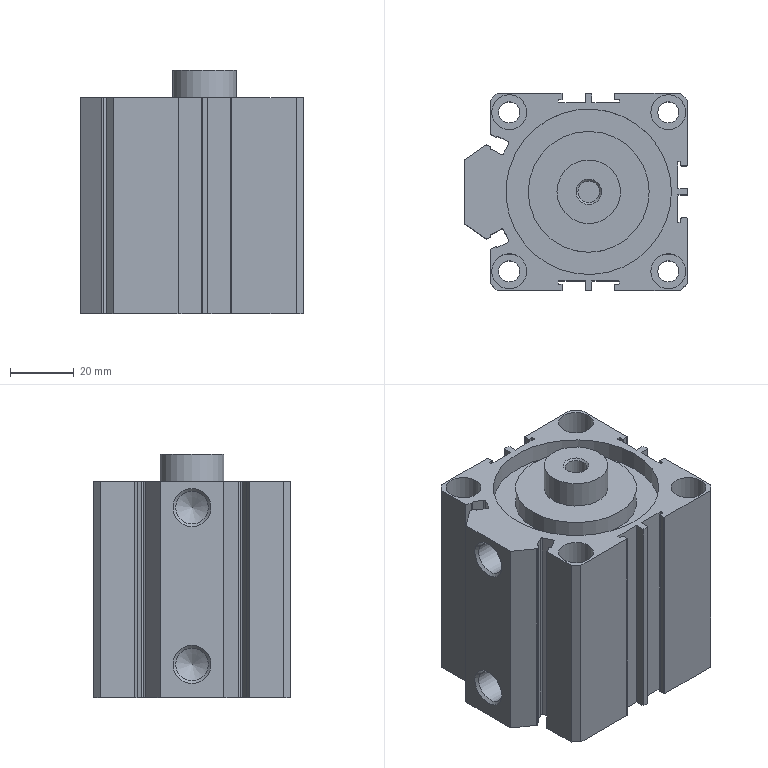Part | NX | features EXTRUDE 7, DATUM_CSYS 5, SKETCH 4, SIMPLE HOLE 3, SYMBOLIC_THREAD 3, HOLE PACKAGE 2 | 2 solids | 142 faces | box 70 x 62 x 76.6 mm | volume 239161 mm3 | plane 73 | cylinder 63 | cone 6 | commonest cylinder face diameters 0.4 x34 0.8 x10 11 x8 6.647 x4 10.3 x2 6.8 x1